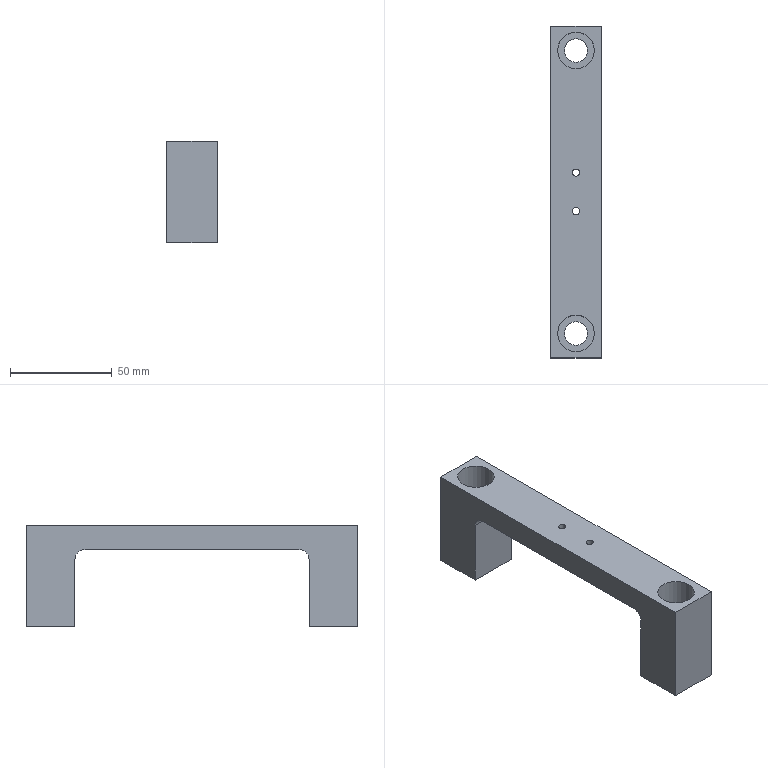Part | NX | features DIE-86 2 | 1 solid | 22 faces | box 25 x 162.999 x 50 mm | volume 78126 mm3 | plane 12 | cylinder 8 | cone 2 | commonest cylinder face diameters 3.5 x2 10 x2 11.5 x2 18 x2
STEP:
#1=CARTESIAN_POINT('',(4239.094,-915.622,853.716));
#2=VERTEX_POINT('',#1);
#3=CARTESIAN_POINT('',(4239.094,-915.622,886.716));
#4=VERTEX_POINT('',#3);
#5=CARTESIAN_POINT('',(4239.094,-915.622,841.716));
#6=DIRECTION('',(0.,0.,-1.));
#7=VECTOR('',#6,1000.);
#8=LINE('',#5,#7);
#9=EDGE_CURVE('',#2,#4,#8,.F.);
#10=ORIENTED_EDGE('',*,*,#9,.T.);
#11=CARTESIAN_POINT('',(4264.094,-915.622,886.716));
#12=VERTEX_POINT('',#11);
#13=CARTESIAN_POINT('',(4264.094,-915.622,886.716));
#14=DIRECTION('',(-1.,0.,0.));
#15=VECTOR('',#14,1000.);
#16=LINE('',#13,#15);
#17=EDGE_CURVE('',#4,#12,#16,.F.);
#18=ORIENTED_EDGE('',*,*,#17,.T.);
#19=CARTESIAN_POINT('',(4264.094,-915.622,853.716));
#20=VERTEX_POINT('',#19);
#21=CARTESIAN_POINT('',(4264.094,-915.622,841.716));
#22=DIRECTION('',(0.,0.,-1.));
#23=VECTOR('',#22,1000.);
#24=LINE('',#21,#23);
#25=EDGE_CURVE('',#20,#12,#24,.F.);
#26=ORIENTED_EDGE('',*,*,#25,.F.);
#27=CARTESIAN_POINT('',(4239.094,-915.622,853.716));
#28=DIRECTION('',(1.,0.,0.));
#29=VECTOR('',#28,1000.);
#30=LINE('',#27,#29);
#31=EDGE_CURVE('',#20,#2,#30,.F.);
#32=ORIENTED_EDGE('',*,*,#31,.T.);
#33=EDGE_LOOP('',(#10,#18,#26,#32));
#34=FACE_BOUND('',#33,.T.);
#35=CARTESIAN_POINT('',(4239.094,-915.622,841.716));
#36=DIRECTION('',(0.,-1.,0.));
#37=DIRECTION('',(0.,0.,-1.));
#38=AXIS2_PLACEMENT_3D('',#35,#36,#37);
#39=PLANE('',#38);
#40=ADVANCED_FACE('',(#34),#39,.F.);
#41=CARTESIAN_POINT('',(4253.344,-867.622,903.716));
#42=VERTEX_POINT('',#41);
#43=CARTESIAN_POINT('',(4251.594,-867.622,903.716));
#44=DIRECTION('',(0.,0.,1.));
#45=DIRECTION('',(1.,0.,0.));
#46=AXIS2_PLACEMENT_3D('',#43,#44,#45);
#47=CIRCLE('',#46,1.75);
#48=EDGE_CURVE('',#42,#42,#47,.F.);
#49=ORIENTED_EDGE('',*,*,#48,.T.);
#50=EDGE_LOOP('',(#49));
#51=FACE_BOUND('',#50,.T.);
#52=CARTESIAN_POINT('',(4253.344,-848.622,903.716));
#53=VERTEX_POINT('',#52);
#54=CARTESIAN_POINT('',(4251.594,-848.622,903.716));
#55=DIRECTION('',(0.,0.,1.));
#56=DIRECTION('',(1.,0.,0.));
#57=AXIS2_PLACEMENT_3D('',#54,#55,#56);
#58=CIRCLE('',#57,1.75);
#59=EDGE_CURVE('',#53,#53,#58,.F.);
#60=ORIENTED_EDGE('',*,*,#59,.T.);
#61=EDGE_LOOP('',(#60));
#62=FACE_BOUND('',#61,.T.);
#63=CARTESIAN_POINT('',(4260.594,-788.623,903.716));
#64=VERTEX_POINT('',#63);
#65=CARTESIAN_POINT('',(4251.594,-788.623,903.716));
#66=DIRECTION('',(0.,0.,1.));
#67=DIRECTION('',(1.,0.,0.));
#68=AXIS2_PLACEMENT_3D('',#65,#66,#67);
#69=CIRCLE('',#68,9.);
#70=EDGE_CURVE('',#64,#64,#69,.F.);
#71=ORIENTED_EDGE('',*,*,#70,.T.);
#72=EDGE_LOOP('',(#71));
#73=FACE_BOUND('',#72,.T.);
#74=CARTESIAN_POINT('',(4260.594,-927.622,903.716));
#75=VERTEX_POINT('',#74);
#76=CARTESIAN_POINT('',(4251.594,-927.622,903.716));
#77=DIRECTION('',(0.,0.,1.));
#78=DIRECTION('',(1.,0.,0.));
#79=AXIS2_PLACEMENT_3D('',#76,#77,#78);
#80=CIRCLE('',#79,9.);
#81=EDGE_CURVE('',#75,#75,#80,.F.);
#82=ORIENTED_EDGE('',*,*,#81,.T.);
#83=EDGE_LOOP('',(#82));
#84=FACE_BOUND('',#83,.T.);
#85=CARTESIAN_POINT('',(4264.094,-776.623,903.716));
#86=VERTEX_POINT('',#85);
#87=CARTESIAN_POINT('',(4264.094,-939.622,903.716));
#88=VERTEX_POINT('',#87);
#89=CARTESIAN_POINT('',(4264.094,-922.622,903.716));
#90=DIRECTION('',(0.,1.,0.));
#91=VECTOR('',#90,1000.);
#92=LINE('',#89,#91);
#93=EDGE_CURVE('',#86,#88,#92,.F.);
#94=ORIENTED_EDGE('',*,*,#93,.F.);
#95=CARTESIAN_POINT('',(4239.094,-776.623,903.716));
#96=VERTEX_POINT('',#95);
#97=CARTESIAN_POINT('',(4239.094,-776.623,903.716));
#98=DIRECTION('',(1.,0.,0.));
#99=VECTOR('',#98,1000.);
#100=LINE('',#97,#99);
#101=EDGE_CURVE('',#96,#86,#100,.T.);
#102=ORIENTED_EDGE('',*,*,#101,.F.);
#103=CARTESIAN_POINT('',(4239.094,-939.622,903.716));
#104=VERTEX_POINT('',#103);
#105=CARTESIAN_POINT('',(4239.094,-922.622,903.716));
#106=DIRECTION('',(0.,1.,0.));
#107=VECTOR('',#106,1000.);
#108=LINE('',#105,#107);
#109=EDGE_CURVE('',#96,#104,#108,.F.);
#110=ORIENTED_EDGE('',*,*,#109,.T.);
#111=CARTESIAN_POINT('',(4239.094,-939.622,903.716));
#112=DIRECTION('',(-1.,0.,0.));
#113=VECTOR('',#112,1000.);
#114=LINE('',#111,#113);
#115=EDGE_CURVE('',#88,#104,#114,.T.);
#116=ORIENTED_EDGE('',*,*,#115,.F.);
#117=EDGE_LOOP('',(#94,#102,#110,#116));
#118=FACE_BOUND('',#117,.T.);
#119=CARTESIAN_POINT('',(4239.094,-922.622,903.716));
#120=DIRECTION('',(0.,0.,1.));
#121=DIRECTION('',(0.,-1.,0.));
#122=AXIS2_PLACEMENT_3D('',#119,#120,#121);
#123=PLANE('',#122);
#124=ADVANCED_FACE('',(#51,#62,#73,#84,#118),#123,.T.);
#125=CARTESIAN_POINT('',(4264.094,-939.622,853.716));
#126=VERTEX_POINT('',#125);
#127=CARTESIAN_POINT('',(4264.094,-939.622,841.716));
#128=DIRECTION('',(0.,0.,-1.));
#129=VECTOR('',#128,1000.);
#130=LINE('',#127,#129);
#131=EDGE_CURVE('',#88,#126,#130,.T.);
#132=ORIENTED_EDGE('',*,*,#131,.F.);
#133=ORIENTED_EDGE('',*,*,#115,.T.);
#134=CARTESIAN_POINT('',(4239.094,-939.622,853.716));
#135=VERTEX_POINT('',#134);
#136=CARTESIAN_POINT('',(4239.094,-939.622,841.716));
#137=DIRECTION('',(0.,0.,-1.));
#138=VECTOR('',#137,1000.);
#139=LINE('',#136,#138);
#140=EDGE_CURVE('',#104,#135,#139,.T.);
#141=ORIENTED_EDGE('',*,*,#140,.T.);
#142=CARTESIAN_POINT('',(4239.094,-939.622,853.716));
#143=DIRECTION('',(1.,0.,0.));
#144=VECTOR('',#143,1000.);
#145=LINE('',#142,#144);
#146=EDGE_CURVE('',#126,#135,#145,.F.);
#147=ORIENTED_EDGE('',*,*,#146,.F.);
#148=EDGE_LOOP('',(#132,#133,#141,#147));
#149=FACE_BOUND('',#148,.T.);
#150=CARTESIAN_POINT('',(4239.094,-939.622,841.716));
#151=DIRECTION('',(0.,1.,0.));
#152=DIRECTION('',(0.,0.,1.));
#153=AXIS2_PLACEMENT_3D('',#150,#151,#152);
#154=PLANE('',#153);
#155=ADVANCED_FACE('',(#149),#154,.F.);
#156=CARTESIAN_POINT('',(4245.844,-927.622,853.716));
#157=VERTEX_POINT('',#156);
#158=CARTESIAN_POINT('',(4251.594,-927.622,853.716));
#159=DIRECTION('',(0.,0.,-1.));
#160=DIRECTION('',(-1.,0.,0.));
#161=AXIS2_PLACEMENT_3D('',#158,#159,#160);
#162=CIRCLE('',#161,5.75);
#163=EDGE_CURVE('',#157,#157,#162,.F.);
#164=ORIENTED_EDGE('',*,*,#163,.T.);
#165=EDGE_LOOP('',(#164));
#166=FACE_BOUND('',#165,.T.);
#167=ORIENTED_EDGE('',*,*,#146,.T.);
#168=CARTESIAN_POINT('',(4239.094,-922.622,853.716));
#169=DIRECTION('',(0.,1.,0.));
#170=VECTOR('',#169,1000.);
#171=LINE('',#168,#170);
#172=EDGE_CURVE('',#135,#2,#171,.T.);
#173=ORIENTED_EDGE('',*,*,#172,.T.);
#174=ORIENTED_EDGE('',*,*,#31,.F.);
#175=CARTESIAN_POINT('',(4264.094,-922.622,853.716));
#176=DIRECTION('',(0.,1.,0.));
#177=VECTOR('',#176,1000.);
#178=LINE('',#175,#177);
#179=EDGE_CURVE('',#126,#20,#178,.T.);
#180=ORIENTED_EDGE('',*,*,#179,.F.);
#181=EDGE_LOOP('',(#167,#173,#174,#180));
#182=FACE_BOUND('',#181,.T.);
#183=CARTESIAN_POINT('',(4239.094,-922.622,853.716));
#184=DIRECTION('',(0.,0.,-1.));
#185=DIRECTION('',(0.,1.,0.));
#186=AXIS2_PLACEMENT_3D('',#183,#184,#185);
#187=PLANE('',#186);
#188=ADVANCED_FACE('',(#166,#182),#187,.T.);
#189=ORIENTED_EDGE('',*,*,#109,.F.);
#190=CARTESIAN_POINT('',(4239.094,-776.623,853.716));
#191=VERTEX_POINT('',#190);
#192=CARTESIAN_POINT('',(4239.094,-776.623,841.716));
#193=DIRECTION('',(0.,0.,-1.));
#194=VECTOR('',#193,1000.);
#195=LINE('',#192,#194);
#196=EDGE_CURVE('',#96,#191,#195,.T.);
#197=ORIENTED_EDGE('',*,*,#196,.T.);
#198=CARTESIAN_POINT('',(4239.094,-800.623,853.716));
#199=VERTEX_POINT('',#198);
#200=CARTESIAN_POINT('',(4239.094,-793.623,853.716));
#201=DIRECTION('',(0.,-1.,0.));
#202=VECTOR('',#201,1000.);
#203=LINE('',#200,#202);
#204=EDGE_CURVE('',#191,#199,#203,.T.);
#205=ORIENTED_EDGE('',*,*,#204,.T.);
#206=CARTESIAN_POINT('',(4239.094,-800.623,886.716));
#207=VERTEX_POINT('',#206);
#208=CARTESIAN_POINT('',(4239.094,-800.623,841.716));
#209=DIRECTION('',(0.,0.,-1.));
#210=VECTOR('',#209,1000.);
#211=LINE('',#208,#210);
#212=EDGE_CURVE('',#199,#207,#211,.F.);
#213=ORIENTED_EDGE('',*,*,#212,.T.);
#214=CARTESIAN_POINT('',(4239.094,-805.623,891.716));
#215=VERTEX_POINT('',#214);
#216=CARTESIAN_POINT('',(4239.094,-805.623,886.716));
#217=DIRECTION('',(1.,0.,0.));
#218=DIRECTION('',(0.,0.,-1.));
#219=AXIS2_PLACEMENT_3D('',#216,#217,#218);
#220=CIRCLE('',#219,5.);
#221=EDGE_CURVE('',#207,#215,#220,.T.);
#222=ORIENTED_EDGE('',*,*,#221,.T.);
#223=CARTESIAN_POINT('',(4239.094,-910.622,891.716));
#224=VERTEX_POINT('',#223);
#225=CARTESIAN_POINT('',(4239.094,-865.622,891.716));
#226=DIRECTION('',(0.,1.,0.));
#227=VECTOR('',#226,1000.);
#228=LINE('',#225,#227);
#229=EDGE_CURVE('',#224,#215,#228,.T.);
#230=ORIENTED_EDGE('',*,*,#229,.F.);
#231=CARTESIAN_POINT('',(4239.094,-910.622,886.716));
#232=DIRECTION('',(1.,0.,0.));
#233=DIRECTION('',(0.,0.,-1.));
#234=AXIS2_PLACEMENT_3D('',#231,#232,#233);
#235=CIRCLE('',#234,5.);
#236=EDGE_CURVE('',#224,#4,#235,.T.);
#237=ORIENTED_EDGE('',*,*,#236,.T.);
#238=ORIENTED_EDGE('',*,*,#9,.F.);
#239=ORIENTED_EDGE('',*,*,#172,.F.);
#240=ORIENTED_EDGE('',*,*,#140,.F.);
#241=EDGE_LOOP('',(#189,#197,#205,#213,#222,#230,#237,#238,#239,#240));
#242=FACE_BOUND('',#241,.T.);
#243=CARTESIAN_POINT('',(4239.094,-922.622,841.716));
#244=DIRECTION('',(1.,0.,0.));
#245=DIRECTION('',(0.,0.,-1.));
#246=AXIS2_PLACEMENT_3D('',#243,#244,#245);
#247=PLANE('',#246);
#248=ADVANCED_FACE('',(#242),#247,.F.);
#249=CARTESIAN_POINT('',(4264.094,-776.623,853.716));
#250=VERTEX_POINT('',#249);
#251=CARTESIAN_POINT('',(4264.094,-776.623,841.716));
#252=DIRECTION('',(0.,0.,-1.));
#253=VECTOR('',#252,1000.);
#254=LINE('',#251,#253);
#255=EDGE_CURVE('',#86,#250,#254,.T.);
#256=ORIENTED_EDGE('',*,*,#255,.F.);
#257=ORIENTED_EDGE('',*,*,#93,.T.);
#258=ORIENTED_EDGE('',*,*,#131,.T.);
#259=ORIENTED_EDGE('',*,*,#179,.T.);
#260=ORIENTED_EDGE('',*,*,#25,.T.);
#261=CARTESIAN_POINT('',(4264.094,-910.622,891.716));
#262=VERTEX_POINT('',#261);
#263=CARTESIAN_POINT('',(4264.094,-910.622,886.716));
#264=DIRECTION('',(1.,0.,0.));
#265=DIRECTION('',(0.,0.,-1.));
#266=AXIS2_PLACEMENT_3D('',#263,#264,#265);
#267=CIRCLE('',#266,5.);
#268=EDGE_CURVE('',#12,#262,#267,.F.);
#269=ORIENTED_EDGE('',*,*,#268,.T.);
#270=CARTESIAN_POINT('',(4264.094,-805.623,891.716));
#271=VERTEX_POINT('',#270);
#272=CARTESIAN_POINT('',(4264.094,-922.622,891.716));
#273=DIRECTION('',(0.,-1.,0.));
#274=VECTOR('',#273,1000.);
#275=LINE('',#272,#274);
#276=EDGE_CURVE('',#271,#262,#275,.T.);
#277=ORIENTED_EDGE('',*,*,#276,.F.);
#278=CARTESIAN_POINT('',(4264.094,-800.623,886.716));
#279=VERTEX_POINT('',#278);
#280=CARTESIAN_POINT('',(4264.094,-805.623,886.716));
#281=DIRECTION('',(1.,0.,0.));
#282=DIRECTION('',(0.,0.,-1.));
#283=AXIS2_PLACEMENT_3D('',#280,#281,#282);
#284=CIRCLE('',#283,5.);
#285=EDGE_CURVE('',#271,#279,#284,.F.);
#286=ORIENTED_EDGE('',*,*,#285,.T.);
#287=CARTESIAN_POINT('',(4264.094,-800.623,853.716));
#288=VERTEX_POINT('',#287);
#289=CARTESIAN_POINT('',(4264.094,-800.623,841.716));
#290=DIRECTION('',(0.,0.,-1.));
#291=VECTOR('',#290,1000.);
#292=LINE('',#289,#291);
#293=EDGE_CURVE('',#288,#279,#292,.F.);
#294=ORIENTED_EDGE('',*,*,#293,.F.);
#295=CARTESIAN_POINT('',(4264.094,-793.623,853.716));
#296=DIRECTION('',(0.,-1.,0.));
#297=VECTOR('',#296,1000.);
#298=LINE('',#295,#297);
#299=EDGE_CURVE('',#250,#288,#298,.T.);
#300=ORIENTED_EDGE('',*,*,#299,.F.);
#301=EDGE_LOOP('',(#256,#257,#258,#259,#260,#269,#277,#286,#294,#300));
#302=FACE_BOUND('',#301,.T.);
#303=CARTESIAN_POINT('',(4264.094,-922.622,841.716));
#304=DIRECTION('',(1.,0.,0.));
#305=DIRECTION('',(0.,0.,-1.));
#306=AXIS2_PLACEMENT_3D('',#303,#304,#305);
#307=PLANE('',#306);
#308=ADVANCED_FACE('',(#302),#307,.T.);
#309=CARTESIAN_POINT('',(4249.594,-867.622,891.716));
#310=VERTEX_POINT('',#309);
#311=CARTESIAN_POINT('',(4251.594,-867.622,891.716));
#312=DIRECTION('',(0.,0.,-1.));
#313=DIRECTION('',(-1.,0.,0.));
#314=AXIS2_PLACEMENT_3D('',#311,#312,#313);
#315=CIRCLE('',#314,2.);
#316=EDGE_CURVE('',#310,#310,#315,.T.);
#317=ORIENTED_EDGE('',*,*,#316,.F.);
#318=EDGE_LOOP('',(#317));
#319=FACE_BOUND('',#318,.T.);
#320=CARTESIAN_POINT('',(4249.594,-848.622,891.716));
#321=VERTEX_POINT('',#320);
#322=CARTESIAN_POINT('',(4251.594,-848.622,891.716));
#323=DIRECTION('',(0.,0.,-1.));
#324=DIRECTION('',(-1.,0.,0.));
#325=AXIS2_PLACEMENT_3D('',#322,#323,#324);
#326=CIRCLE('',#325,2.);
#327=EDGE_CURVE('',#321,#321,#326,.T.);
#328=ORIENTED_EDGE('',*,*,#327,.F.);
#329=EDGE_LOOP('',(#328));
#330=FACE_BOUND('',#329,.T.);
#331=ORIENTED_EDGE('',*,*,#276,.T.);
#332=CARTESIAN_POINT('',(4239.094,-910.622,891.716));
#333=DIRECTION('',(-1.,0.,0.));
#334=VECTOR('',#333,1000.);
#335=LINE('',#332,#334);
#336=EDGE_CURVE('',#262,#224,#335,.T.);
#337=ORIENTED_EDGE('',*,*,#336,.T.);
#338=ORIENTED_EDGE('',*,*,#229,.T.);
#339=CARTESIAN_POINT('',(4264.094,-805.623,891.716));
#340=DIRECTION('',(-1.,0.,0.));
#341=VECTOR('',#340,1000.);
#342=LINE('',#339,#341);
#343=EDGE_CURVE('',#215,#271,#342,.F.);
#344=ORIENTED_EDGE('',*,*,#343,.T.);
#345=EDGE_LOOP('',(#331,#337,#338,#344));
#346=FACE_BOUND('',#345,.T.);
#347=CARTESIAN_POINT('',(4251.594,-865.622,891.716));
#348=DIRECTION('',(0.,0.,1.));
#349=DIRECTION('',(1.,0.,0.));
#350=AXIS2_PLACEMENT_3D('',#347,#348,#349);
#351=PLANE('',#350);
#352=ADVANCED_FACE('',(#319,#330,#346),#351,.F.);
#353=ORIENTED_EDGE('',*,*,#293,.T.);
#354=CARTESIAN_POINT('',(4239.094,-800.623,886.716));
#355=DIRECTION('',(-1.,0.,0.));
#356=VECTOR('',#355,1000.);
#357=LINE('',#354,#356);
#358=EDGE_CURVE('',#279,#207,#357,.T.);
#359=ORIENTED_EDGE('',*,*,#358,.T.);
#360=ORIENTED_EDGE('',*,*,#212,.F.);
#361=CARTESIAN_POINT('',(4239.094,-800.623,853.716));
#362=DIRECTION('',(1.,0.,0.));
#363=VECTOR('',#362,1000.);
#364=LINE('',#361,#363);
#365=EDGE_CURVE('',#288,#199,#364,.F.);
#366=ORIENTED_EDGE('',*,*,#365,.F.);
#367=EDGE_LOOP('',(#353,#359,#360,#366));
#368=FACE_BOUND('',#367,.T.);
#369=CARTESIAN_POINT('',(4239.094,-800.623,841.716));
#370=DIRECTION('',(0.,1.,0.));
#371=DIRECTION('',(0.,0.,-1.));
#372=AXIS2_PLACEMENT_3D('',#369,#370,#371);
#373=PLANE('',#372);
#374=ADVANCED_FACE('',(#368),#373,.F.);
#375=ORIENTED_EDGE('',*,*,#196,.F.);
#376=ORIENTED_EDGE('',*,*,#101,.T.);
#377=ORIENTED_EDGE('',*,*,#255,.T.);
#378=CARTESIAN_POINT('',(4239.094,-776.623,853.716));
#379=DIRECTION('',(1.,0.,0.));
#380=VECTOR('',#379,1000.);
#381=LINE('',#378,#380);
#382=EDGE_CURVE('',#250,#191,#381,.F.);
#383=ORIENTED_EDGE('',*,*,#382,.T.);
#384=EDGE_LOOP('',(#375,#376,#377,#383));
#385=FACE_BOUND('',#384,.T.);
#386=CARTESIAN_POINT('',(4239.094,-776.623,841.716));
#387=DIRECTION('',(0.,-1.,0.));
#388=DIRECTION('',(0.,0.,1.));
#389=AXIS2_PLACEMENT_3D('',#386,#387,#388);
#390=PLANE('',#389);
#391=ADVANCED_FACE('',(#385),#390,.F.);
#392=CARTESIAN_POINT('',(4245.844,-788.623,853.716));
#393=VERTEX_POINT('',#392);
#394=CARTESIAN_POINT('',(4251.594,-788.623,853.716));
#395=DIRECTION('',(0.,0.,-1.));
#396=DIRECTION('',(-1.,0.,0.));
#397=AXIS2_PLACEMENT_3D('',#394,#395,#396);
#398=CIRCLE('',#397,5.75);
#399=EDGE_CURVE('',#393,#393,#398,.F.);
#400=ORIENTED_EDGE('',*,*,#399,.T.);
#401=EDGE_LOOP('',(#400));
#402=FACE_BOUND('',#401,.T.);
#403=ORIENTED_EDGE('',*,*,#382,.F.);
#404=ORIENTED_EDGE('',*,*,#299,.T.);
#405=ORIENTED_EDGE('',*,*,#365,.T.);
#406=ORIENTED_EDGE('',*,*,#204,.F.);
#407=EDGE_LOOP('',(#403,#404,#405,#406));
#408=FACE_BOUND('',#407,.T.);
#409=CARTESIAN_POINT('',(4239.094,-793.623,853.716));
#410=DIRECTION('',(0.,0.,-1.));
#411=DIRECTION('',(0.,-1.,0.));
#412=AXIS2_PLACEMENT_3D('',#409,#410,#411);
#413=PLANE('',#412);
#414=ADVANCED_FACE('',(#402,#408),#413,.T.);
#415=CARTESIAN_POINT('',(4257.344,-927.622,883.716));
#416=VERTEX_POINT('',#415);
#417=CARTESIAN_POINT('',(4251.594,-927.622,883.716));
#418=DIRECTION('',(0.,0.,1.));
#419=DIRECTION('',(1.,0.,0.));
#420=AXIS2_PLACEMENT_3D('',#417,#418,#419);
#421=CIRCLE('',#420,5.75);
#422=EDGE_CURVE('',#416,#416,#421,.T.);
#423=ORIENTED_EDGE('',*,*,#422,.T.);
#424=EDGE_LOOP('',(#423));
#425=FACE_BOUND('',#424,.T.);
#426=ORIENTED_EDGE('',*,*,#163,.F.);
#427=EDGE_LOOP('',(#426));
#428=FACE_BOUND('',#427,.T.);
#429=CARTESIAN_POINT('',(4251.594,-927.622,852.716));
#430=DIRECTION('',(0.,0.,1.));
#431=DIRECTION('',(1.,0.,0.));
#432=AXIS2_PLACEMENT_3D('',#429,#430,#431);
#433=CYLINDRICAL_SURFACE('',#432,5.75);
#434=ADVANCED_FACE('',(#425,#428),#433,.F.);
#435=CARTESIAN_POINT('',(4260.594,-927.622,883.716));
#436=VERTEX_POINT('',#435);
#437=CARTESIAN_POINT('',(4251.594,-927.622,883.716));
#438=DIRECTION('',(0.,0.,1.));
#439=DIRECTION('',(1.,0.,0.));
#440=AXIS2_PLACEMENT_3D('',#437,#438,#439);
#441=CIRCLE('',#440,9.);
#442=EDGE_CURVE('',#436,#436,#441,.F.);
#443=ORIENTED_EDGE('',*,*,#442,.T.);
#444=EDGE_LOOP('',(#443));
#445=FACE_BOUND('',#444,.T.);
#446=ORIENTED_EDGE('',*,*,#81,.F.);
#447=EDGE_LOOP('',(#446));
#448=FACE_BOUND('',#447,.T.);
#449=CARTESIAN_POINT('',(4251.594,-927.622,883.716));
#450=DIRECTION('',(0.,0.,1.));
#451=DIRECTION('',(1.,0.,0.));
#452=AXIS2_PLACEMENT_3D('',#449,#450,#451);
#453=CYLINDRICAL_SURFACE('',#452,9.);
#454=ADVANCED_FACE('',(#445,#448),#453,.F.);
#455=ORIENTED_EDGE('',*,*,#422,.F.);
#456=EDGE_LOOP('',(#455));
#457=FACE_BOUND('',#456,.T.);
#458=ORIENTED_EDGE('',*,*,#442,.F.);
#459=EDGE_LOOP('',(#458));
#460=FACE_BOUND('',#459,.T.);
#461=CARTESIAN_POINT('',(4251.594,-927.622,883.716));
#462=DIRECTION('',(0.,0.,1.));
#463=DIRECTION('',(1.,0.,0.));
#464=AXIS2_PLACEMENT_3D('',#461,#462,#463);
#465=PLANE('',#464);
#466=ADVANCED_FACE('',(#457,#460),#465,.T.);
#467=CARTESIAN_POINT('',(4257.344,-788.623,883.716));
#468=VERTEX_POINT('',#467);
#469=CARTESIAN_POINT('',(4251.594,-788.623,883.716));
#470=DIRECTION('',(0.,0.,-1.));
#471=DIRECTION('',(1.,0.,0.));
#472=AXIS2_PLACEMENT_3D('',#469,#470,#471);
#473=CIRCLE('',#472,5.75);
#474=EDGE_CURVE('',#468,#468,#473,.T.);
#475=ORIENTED_EDGE('',*,*,#474,.F.);
#476=EDGE_LOOP('',(#475));
#477=FACE_BOUND('',#476,.T.);
#478=ORIENTED_EDGE('',*,*,#399,.F.);
#479=EDGE_LOOP('',(#478));
#480=FACE_BOUND('',#479,.T.);
#481=CARTESIAN_POINT('',(4251.594,-788.623,852.716));
#482=DIRECTION('',(0.,0.,1.));
#483=DIRECTION('',(1.,0.,0.));
#484=AXIS2_PLACEMENT_3D('',#481,#482,#483);
#485=CYLINDRICAL_SURFACE('',#484,5.75);
#486=ADVANCED_FACE('',(#477,#480),#485,.F.);
#487=CARTESIAN_POINT('',(4260.594,-788.623,883.716));
#488=VERTEX_POINT('',#487);
#489=CARTESIAN_POINT('',(4251.594,-788.623,883.716));
#490=DIRECTION('',(0.,0.,-1.));
#491=DIRECTION('',(1.,0.,0.));
#492=AXIS2_PLACEMENT_3D('',#489,#490,#491);
#493=CIRCLE('',#492,9.);
#494=EDGE_CURVE('',#488,#488,#493,.F.);
#495=ORIENTED_EDGE('',*,*,#494,.F.);
#496=EDGE_LOOP('',(#495));
#497=FACE_BOUND('',#496,.T.);
#498=ORIENTED_EDGE('',*,*,#70,.F.);
#499=EDGE_LOOP('',(#498));
#500=FACE_BOUND('',#499,.T.);
#501=CARTESIAN_POINT('',(4251.594,-788.623,883.716));
#502=DIRECTION('',(0.,0.,1.));
#503=DIRECTION('',(1.,0.,0.));
#504=AXIS2_PLACEMENT_3D('',#501,#502,#503);
#505=CYLINDRICAL_SURFACE('',#504,9.);
#506=ADVANCED_FACE('',(#497,#500),#505,.F.);
#507=ORIENTED_EDGE('',*,*,#474,.T.);
#508=EDGE_LOOP('',(#507));
#509=FACE_BOUND('',#508,.T.);
#510=ORIENTED_EDGE('',*,*,#494,.T.);
#511=EDGE_LOOP('',(#510));
#512=FACE_BOUND('',#511,.T.);
#513=CARTESIAN_POINT('',(4251.594,-788.623,883.716));
#514=DIRECTION('',(0.,0.,1.));
#515=DIRECTION('',(1.,0.,0.));
#516=AXIS2_PLACEMENT_3D('',#513,#514,#515);
#517=PLANE('',#516);
#518=ADVANCED_FACE('',(#509,#512),#517,.T.);
#519=ORIENTED_EDGE('',*,*,#268,.F.);
#520=ORIENTED_EDGE('',*,*,#17,.F.);
#521=ORIENTED_EDGE('',*,*,#236,.F.);
#522=ORIENTED_EDGE('',*,*,#336,.F.);
#523=EDGE_LOOP('',(#519,#520,#521,#522));
#524=FACE_BOUND('',#523,.T.);
#525=CARTESIAN_POINT('',(4251.594,-910.622,886.716));
#526=DIRECTION('',(1.,0.,0.));
#527=DIRECTION('',(0.,0.,-1.));
#528=AXIS2_PLACEMENT_3D('',#525,#526,#527);
#529=CYLINDRICAL_SURFACE('',#528,5.);
#530=ADVANCED_FACE('',(#524),#529,.F.);
#531=ORIENTED_EDGE('',*,*,#285,.F.);
#532=ORIENTED_EDGE('',*,*,#343,.F.);
#533=ORIENTED_EDGE('',*,*,#221,.F.);
#534=ORIENTED_EDGE('',*,*,#358,.F.);
#535=EDGE_LOOP('',(#531,#532,#533,#534));
#536=FACE_BOUND('',#535,.T.);
#537=CARTESIAN_POINT('',(4239.094,-805.623,886.716));
#538=DIRECTION('',(1.,0.,0.));
#539=DIRECTION('',(0.,0.,-1.));
#540=AXIS2_PLACEMENT_3D('',#537,#538,#539);
#541=CYLINDRICAL_SURFACE('',#540,5.);
#542=ADVANCED_FACE('',(#536),#541,.F.);
#543=CARTESIAN_POINT('',(4249.844,-867.622,891.966));
#544=VERTEX_POINT('',#543);
#545=CARTESIAN_POINT('',(4251.594,-867.622,891.966));
#546=DIRECTION('',(0.,0.,-1.));
#547=DIRECTION('',(-1.,0.,0.));
#548=AXIS2_PLACEMENT_3D('',#545,#546,#547);
#549=CIRCLE('',#548,1.75);
#550=EDGE_CURVE('',#544,#544,#549,.F.);
#551=ORIENTED_EDGE('',*,*,#550,.F.);
#552=EDGE_LOOP('',(#551));
#553=FACE_BOUND('',#552,.T.);
#554=ORIENTED_EDGE('',*,*,#48,.F.);
#555=EDGE_LOOP('',(#554));
#556=FACE_BOUND('',#555,.T.);
#557=CARTESIAN_POINT('',(4251.594,-867.622,913.466));
#558=DIRECTION('',(0.,0.,-1.));
#559=DIRECTION('',(-1.,0.,0.));
#560=AXIS2_PLACEMENT_3D('',#557,#558,#559);
#561=CYLINDRICAL_SURFACE('',#560,1.75);
#562=ADVANCED_FACE('',(#553,#556),#561,.F.);
#563=ORIENTED_EDGE('',*,*,#550,.T.);
#564=EDGE_LOOP('',(#563));
#565=FACE_BOUND('',#564,.T.);
#566=ORIENTED_EDGE('',*,*,#316,.T.);
#567=EDGE_LOOP('',(#566));
#568=FACE_BOUND('',#567,.T.);
#569=CARTESIAN_POINT('',(4251.594,-867.622,891.716));
#570=DIRECTION('',(0.,0.,-1.));
#571=DIRECTION('',(-1.,0.,0.));
#572=AXIS2_PLACEMENT_3D('',#569,#570,#571);
#573=CONICAL_SURFACE('',#572,2.,0.7854);
#574=ADVANCED_FACE('',(#565,#568),#573,.F.);
#575=ORIENTED_EDGE('',*,*,#59,.F.);
#576=EDGE_LOOP('',(#575));
#577=FACE_BOUND('',#576,.T.);
#578=CARTESIAN_POINT('',(4249.844,-848.622,891.966));
#579=VERTEX_POINT('',#578);
#580=CARTESIAN_POINT('',(4251.594,-848.622,891.966));
#581=DIRECTION('',(0.,0.,-1.));
#582=DIRECTION('',(-1.,0.,0.));
#583=AXIS2_PLACEMENT_3D('',#580,#581,#582);
#584=CIRCLE('',#583,1.75);
#585=EDGE_CURVE('',#579,#579,#584,.F.);
#586=ORIENTED_EDGE('',*,*,#585,.F.);
#587=EDGE_LOOP('',(#586));
#588=FACE_BOUND('',#587,.T.);
#589=CARTESIAN_POINT('',(4251.594,-848.622,913.466));
#590=DIRECTION('',(0.,0.,-1.));
#591=DIRECTION('',(-1.,0.,0.));
#592=AXIS2_PLACEMENT_3D('',#589,#590,#591);
#593=CYLINDRICAL_SURFACE('',#592,1.75);
#594=ADVANCED_FACE('',(#577,#588),#593,.F.);
#595=ORIENTED_EDGE('',*,*,#585,.T.);
#596=EDGE_LOOP('',(#595));
#597=FACE_BOUND('',#596,.T.);
#598=ORIENTED_EDGE('',*,*,#327,.T.);
#599=EDGE_LOOP('',(#598));
#600=FACE_BOUND('',#599,.T.);
#601=CARTESIAN_POINT('',(4251.594,-848.622,891.716));
#602=DIRECTION('',(0.,0.,-1.));
#603=DIRECTION('',(-1.,0.,0.));
#604=AXIS2_PLACEMENT_3D('',#601,#602,#603);
#605=CONICAL_SURFACE('',#604,2.,0.7854);
#606=ADVANCED_FACE('',(#597,#600),#605,.F.);
#607=CLOSED_SHELL('',(#40,#124,#155,#188,#248,#308,#352,#374,#391,#414,#434,#454,#466,#486,#506,#518,#530,#542,#562,#574,#594,#606));
#608=MANIFOLD_SOLID_BREP('',#607);
#609=(LENGTH_UNIT()NAMED_UNIT(*)SI_UNIT(.MILLI.,.METRE.));
#610=UNCERTAINTY_MEASURE_WITH_UNIT(LENGTH_MEASURE(0.00001),#609,'','');
#611=(NAMED_UNIT(*)PLANE_ANGLE_UNIT()SI_UNIT($,.RADIAN.));
#612=(NAMED_UNIT(*)SI_UNIT($,.STERADIAN.)SOLID_ANGLE_UNIT());
#613=(GEOMETRIC_REPRESENTATION_CONTEXT(3)GLOBAL_UNCERTAINTY_ASSIGNED_CONTEXT((#610))GLOBAL_UNIT_ASSIGNED_CONTEXT((#609,#611,#612))REPRESENTATION_CONTEXT('',''));
#614=ADVANCED_BREP_SHAPE_REPRESENTATION('',(#608),#613);